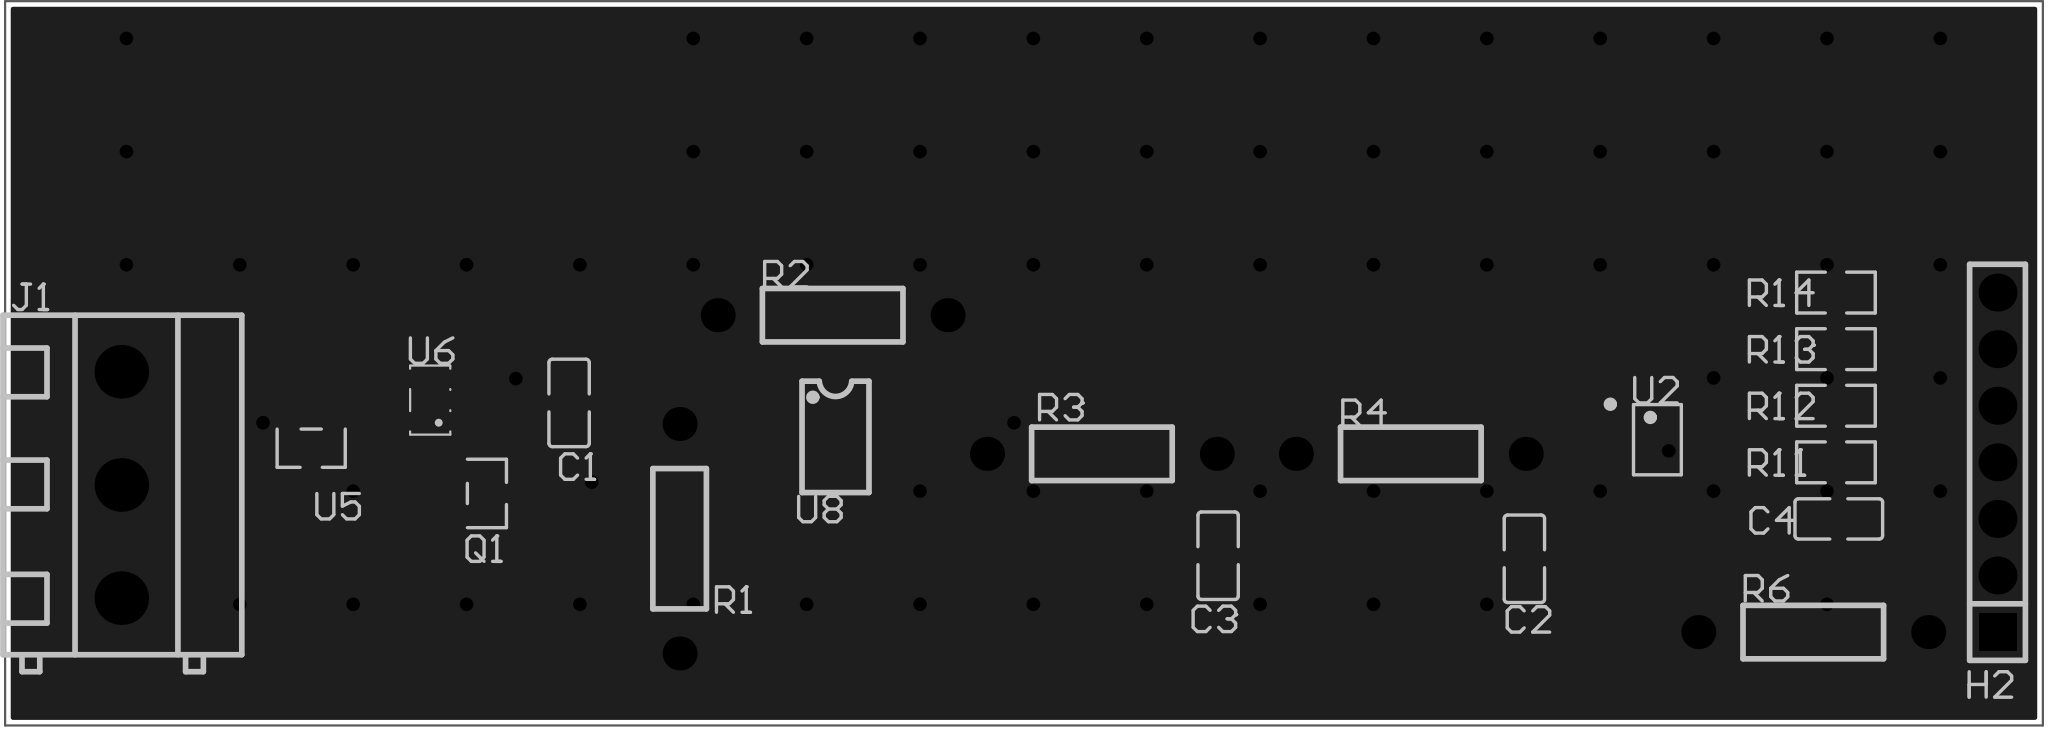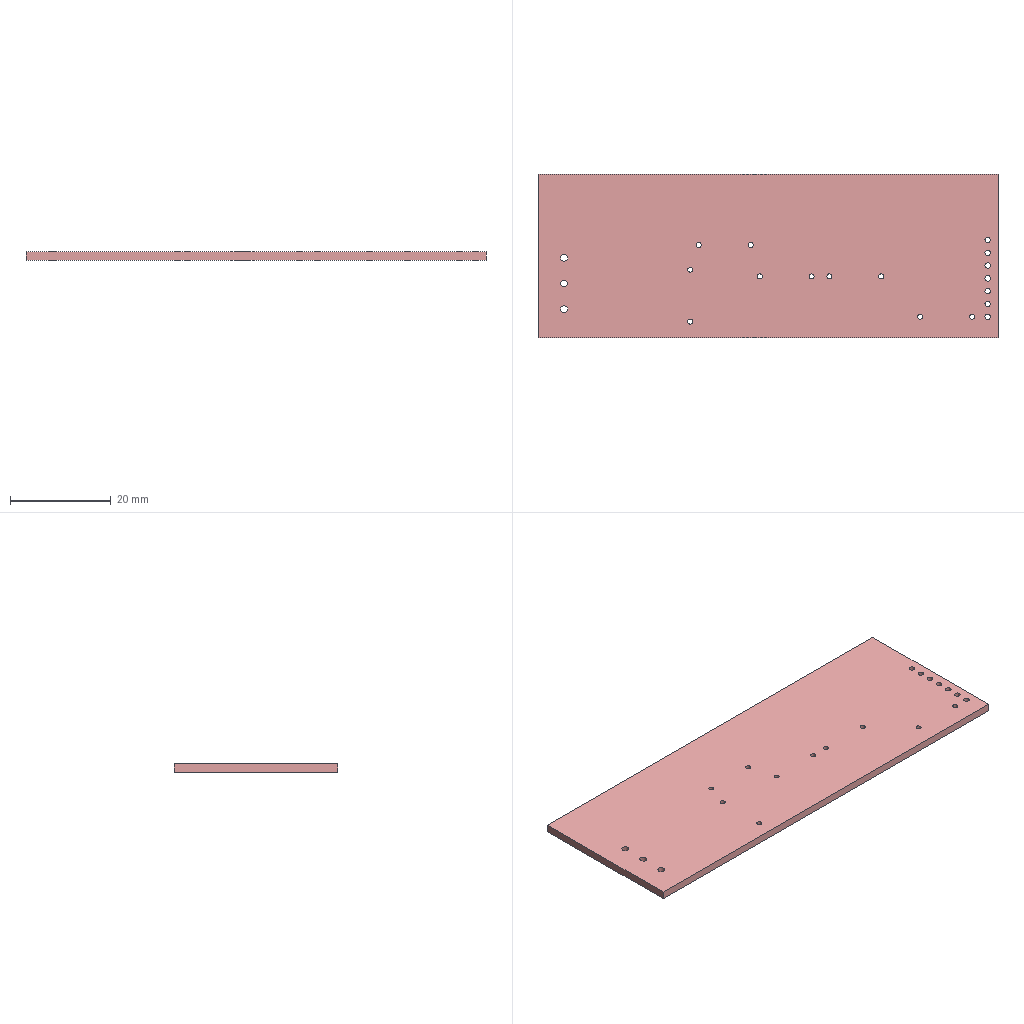Circuit board layout | Altium Designer | box 91.3 x 32.5 x 1.6 mm
Layer stack:
# Altium Designer layer stack of  (unit mm; dielectric type: 0 none, 1 core, 2 prepreg, 3 surface material)
index,name,kind,layer,copper_thickness_mm,dielectric_type,dielectric_thickness_mm,dielectric_material,dielectric_constant
0,Top Paste Mask Layer,other,,,,,,
1,Top Silkscreen Layer,other,,,,,,
2,Top Solder Mask Layer,dielectric,,,3,0.01,,3.3
3,Top Layer,copper,Top Layer,0.035,,,,
4,Dielectric1,dielectric,,,3,1.51,FR4,4.5
5,Bottom Layer,copper,Bottom Layer,0.035,,,,
6,Bottom Solder Mask Layer,dielectric,,,3,0.01,,3.3
7,Bottom Silkscreen Layer,other,,,,,,
8,Bottom Paste Mask Layer,other,,,,,,
# drill layer pairs: low layer,high layer
drill_pair,Top Layer,Bottom Layer
Part placement:
Designator,Comment,Layer,Footprint,Center-X(mm),Center-Y(mm),Rotation
C1,100nF,TopLayer,C0805,133.477,104.521,90
R11,50,TopLayer,R0805,190.246,101.854,0
R12,50,TopLayer,R0805,190.246,104.394,0
R13,50,TopLayer,R0805,190.246,106.934,0
R14,50,TopLayer,R0805,190.246,109.474,0
H2,PZ254V-11-07P,TopLayer,HDR-TH_7P-P2.54-V-M,197.485,101.854,90
J1,KF128-5.08-3P-AA,TopLayer,CONN-TH_3P-P5.08_KF128-5.08-3P,113.411,100.838,270
Q1,2N7002K-T1-GE3,TopLayer,SOT-23-3_L2.9-W1.6-P1.90-LS2.8-BR,129.794,100.457,180
R1,3.3kΩ,TopLayer,Res_1/4W,138.43,98.425,90
R2,3.3kΩ,TopLayer,Res_1/4W,145.288,108.458,0
R3,200,TopLayer,Res_1/4W,157.353,102.235,0
R4,200,TopLayer,Res_1/4W,171.196,102.235,0
R6,10K,TopLayer,Res_1/4W,189.23,94.234,0
U2,GD30AD3344,TopLayer,MSOP-10_L3.0-W3.0-P0.50-LS5.0-BL,182.245,102.87,270
U5,REF3033AIDBZR,TopLayer,SOT-23-3_L3.0-W1.7-P0.95-LS2.9-BR,121.92,102.489,90
C4,100nF,TopLayer,C0805,190.373,99.314,0
C2,100nF,TopLayer,C0805,176.284,97.525,90
C3,100nF,TopLayer,C0805,162.56,97.663,90
U6,OPA333AIDBVR,TopLayer,SOT-23-5_L3.0-W1.7-P0.95-LS2.8-BR,127.254,104.648,0
U8,AD623ARZ-R7,TopLayer,SOIC-8_L5.0-W4.0-P1.27-LS6.0-BL,145.415,102.997,270
Pad and via stacks:
# Altium Designer via and pad stacks of  (unit mm). Each distinct definition once, with the count of objects using it.
# via: kind,start_layer,end_layer,hole_mm,diameter_mm,mode(0 simple;1 top-mid-bottom;2 full stack),diameter_per_layer,count,example_net
# pad: kind,layer,hole_mm,hole_type(0 round;1 square;2 slot),plating,top_size,top_shape(1 round;2 rect;3 octagon;9 rounded rect),mid_size,bottom_size,mode,footprint,size_per_layer,count,example
pad,Top Layer,0,0,plated,1.41x1.35,2,1.41x1.35,1.41x1.35,0,C0805,,8,C1.2
pad,Top Layer,0,0,plated,1.133x1.377,2,1.133x1.377,1.133x1.377,0,R0805,,8,R11.2
pad,Top Layer,0,0,plated,1.07x0.6,2,1.07x0.6,1.07x0.6,0,SOT-23-3_L2.9-W1.6-P1.90-LS2.8-BR,,3,Q1.1
pad,Top Layer,0,0,plated,0.28x1.62,1,0.28x1.62,0.28x1.62,0,MSOP-10_L3.0-W3.0-P0.50-LS5.0-BL,,10,U2.1
pad,Top Layer,0,0,plated,1.038x0.532,2,1.038x0.532,1.038x0.532,0,SOT-23-3_L3.0-W1.7-P0.95-LS2.9-BR,,3,U5.1
pad,Top Layer,0,0,plated,1.1x0.6,2,1.1x0.6,1.1x0.6,0,SOT-23-5_L3.0-W1.7-P0.95-LS2.8-BR,,5,U6.5
pad,Top Layer,0,0,plated,0.5684x1.95,1,0.5684x1.95,0.5684x1.95,0,SOIC-8_L5.0-W4.0-P1.27-LS6.0-BL,,8,U8.1
pad,Multi-Layer,1.1,0,plated,1.7x1.7,2,1.7x1.7,1.7x1.7,0,HDR-TH_7P-P2.54-V-M,,1,H2.1
pad,Multi-Layer,1.1,0,plated,1.7x1.7,1,1.7x1.7,1.7x1.7,0,HDR-TH_7P-P2.54-V-M,,6,H2.2
pad,Multi-Layer,1.4,0,plated,2.4x2.4,1,2.4x2.4,2.4x2.4,0,CONN-TH_3P-P5.08_KF128-5.08-3P,,3,J1.1
pad,Multi-Layer,1,0,plated,1.524x1.524,1,1.524x1.524,1.524x1.524,0,Res_1/4W,,10,R1.1
via,Top Layer,Bottom Layer,0.3048,0.61,0,,75,3.3V
Copper pours:
name,layer,net,type(0 solid;1 hatched;2 none)
Top Layer-AGND,Top Layer,AGND,0
Bottom Layer-AGND,Bottom Layer,AGND,0